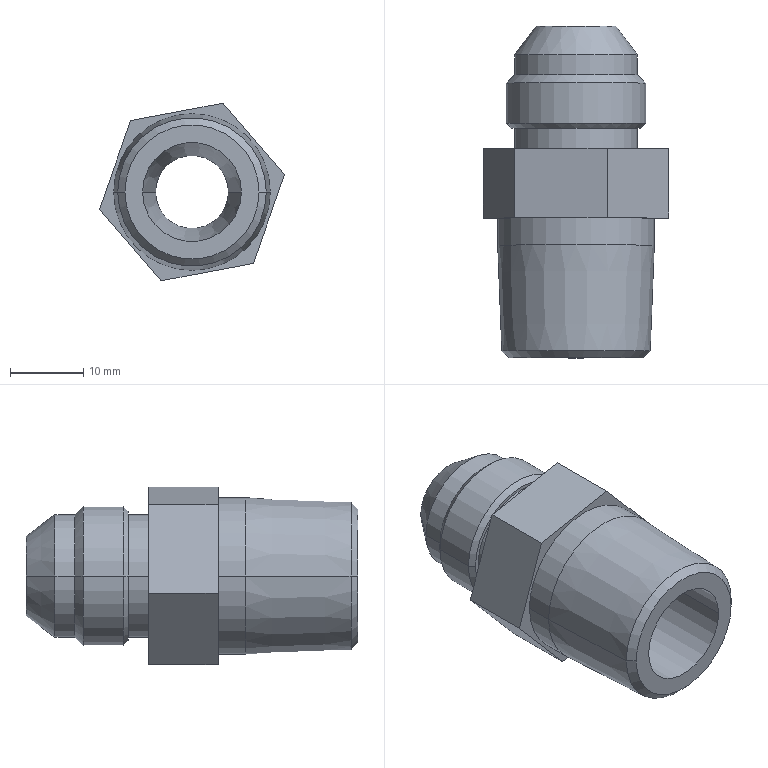Part | STEP file | 4-20.sldasm-Part-131 | 1 solid | 35 faces | box 25.216 x 45.212 x 24.222 mm | volume 9310 mm3 | cone 12 | cylinder 12 | plane 11 | commonest cylinder face diameters 9.931 x2 13.487 x2 16.662 x2 16.739 x2 19.009 x2 21.336 x2
STEP:
#1=CARTESIAN_POINT('',(133.988,509.63,44.));
#2=VERTEX_POINT('',#1);
#3=CARTESIAN_POINT('',(152.262,509.63,44.));
#4=VERTEX_POINT('',#3);
#5=CARTESIAN_POINT('',(143.125,509.63,44.));
#6=DIRECTION('',(0.,-1.,0.));
#7=DIRECTION('',(-1.,0.,0.));
#8=AXIS2_PLACEMENT_3D('',#5,#6,#7);
#9=CIRCLE('',#8,9.137);
#10=EDGE_CURVE('',#2,#4,#9,.T.);
#11=ORIENTED_EDGE('',*,*,#10,.F.);
#12=CARTESIAN_POINT('',(133.012,510.57,44.));
#13=VERTEX_POINT('',#12);
#14=CARTESIAN_POINT('',(133.988,509.63,44.));
#15=DIRECTION('',(-0.7206,0.6934,0.));
#16=VECTOR('',#15,1000.);
#17=LINE('',#14,#16);
#18=EDGE_CURVE('',#2,#13,#17,.T.);
#19=ORIENTED_EDGE('',*,*,#18,.T.);
#20=CARTESIAN_POINT('',(153.238,510.57,44.));
#21=VERTEX_POINT('',#20);
#22=CARTESIAN_POINT('',(143.125,510.57,44.));
#23=DIRECTION('',(0.,1.,0.));
#24=DIRECTION('',(-1.,0.,0.));
#25=AXIS2_PLACEMENT_3D('',#22,#23,#24);
#26=CIRCLE('',#25,10.113);
#27=EDGE_CURVE('',#21,#13,#26,.T.);
#28=ORIENTED_EDGE('',*,*,#27,.F.);
#29=CARTESIAN_POINT('',(152.262,509.63,44.));
#30=DIRECTION('',(0.7206,0.6934,0.));
#31=VECTOR('',#30,1000.);
#32=LINE('',#29,#31);
#33=EDGE_CURVE('',#4,#21,#32,.T.);
#34=ORIENTED_EDGE('',*,*,#33,.F.);
#35=EDGE_LOOP('',(#11,#19,#28,#34));
#36=FACE_OUTER_BOUND('',#35,.T.);
#37=CARTESIAN_POINT('',(143.125,509.63,44.));
#38=DIRECTION('',(0.,1.,0.));
#39=DIRECTION('',(1.,0.,0.));
#40=AXIS2_PLACEMENT_3D('',#37,#38,#39);
#41=CONICAL_SURFACE('',#40,9.137,0.8046);
#42=ADVANCED_FACE('',(#36),#41,.T.);
#43=CARTESIAN_POINT('',(134.756,548.213,44.));
#44=VERTEX_POINT('',#43);
#45=CARTESIAN_POINT('',(151.494,548.213,44.));
#46=VERTEX_POINT('',#45);
#47=CARTESIAN_POINT('',(143.125,548.213,44.));
#48=DIRECTION('',(0.,-1.,0.));
#49=DIRECTION('',(-1.,0.,0.));
#50=AXIS2_PLACEMENT_3D('',#47,#48,#49);
#51=CIRCLE('',#50,8.369);
#52=EDGE_CURVE('',#44,#46,#51,.T.);
#53=ORIENTED_EDGE('',*,*,#52,.T.);
#54=CARTESIAN_POINT('',(152.63,547.078,44.));
#55=VERTEX_POINT('',#54);
#56=CARTESIAN_POINT('',(152.63,547.078,44.));
#57=DIRECTION('',(0.7071,-0.7071,0.));
#58=VECTOR('',#57,1000.);
#59=LINE('',#56,#58);
#60=EDGE_CURVE('',#46,#55,#59,.T.);
#61=ORIENTED_EDGE('',*,*,#60,.T.);
#62=CARTESIAN_POINT('',(133.62,547.078,44.));
#63=VERTEX_POINT('',#62);
#64=CARTESIAN_POINT('',(143.125,547.078,44.));
#65=DIRECTION('',(0.,-1.,0.));
#66=DIRECTION('',(1.,0.,0.));
#67=AXIS2_PLACEMENT_3D('',#64,#65,#66);
#68=CIRCLE('',#67,9.505);
#69=EDGE_CURVE('',#63,#55,#68,.T.);
#70=ORIENTED_EDGE('',*,*,#69,.F.);
#71=CARTESIAN_POINT('',(133.62,547.078,44.));
#72=DIRECTION('',(-0.7071,-0.7071,0.));
#73=VECTOR('',#72,1000.);
#74=LINE('',#71,#73);
#75=EDGE_CURVE('',#44,#63,#74,.T.);
#76=ORIENTED_EDGE('',*,*,#75,.F.);
#77=EDGE_LOOP('',(#53,#61,#70,#76));
#78=FACE_OUTER_BOUND('',#77,.T.);
#79=CARTESIAN_POINT('',(143.125,547.078,44.));
#80=DIRECTION('',(0.,-1.,0.));
#81=DIRECTION('',(-1.,0.,0.));
#82=AXIS2_PLACEMENT_3D('',#79,#80,#81);
#83=CONICAL_SURFACE('',#82,9.505,0.7854);
#84=ADVANCED_FACE('',(#78),#83,.T.);
#85=CARTESIAN_POINT('',(134.298,540.923,44.));
#86=VERTEX_POINT('',#85);
#87=CARTESIAN_POINT('',(151.951,540.923,44.));
#88=VERTEX_POINT('',#87);
#89=CARTESIAN_POINT('',(143.125,540.923,44.));
#90=DIRECTION('',(0.,-1.,0.));
#91=DIRECTION('',(-1.,0.,0.));
#92=AXIS2_PLACEMENT_3D('',#89,#90,#91);
#93=CIRCLE('',#92,8.826);
#94=EDGE_CURVE('',#86,#88,#93,.T.);
#95=ORIENTED_EDGE('',*,*,#94,.F.);
#96=CARTESIAN_POINT('',(133.62,541.601,44.));
#97=VERTEX_POINT('',#96);
#98=CARTESIAN_POINT('',(134.298,540.923,44.));
#99=DIRECTION('',(-0.7071,0.7071,0.));
#100=VECTOR('',#99,1000.);
#101=LINE('',#98,#100);
#102=EDGE_CURVE('',#86,#97,#101,.T.);
#103=ORIENTED_EDGE('',*,*,#102,.T.);
#104=CARTESIAN_POINT('',(152.63,541.601,44.));
#105=VERTEX_POINT('',#104);
#106=CARTESIAN_POINT('',(143.125,541.601,44.));
#107=DIRECTION('',(0.,1.,0.));
#108=DIRECTION('',(-1.,0.,0.));
#109=AXIS2_PLACEMENT_3D('',#106,#107,#108);
#110=CIRCLE('',#109,9.505);
#111=EDGE_CURVE('',#105,#97,#110,.T.);
#112=ORIENTED_EDGE('',*,*,#111,.F.);
#113=CARTESIAN_POINT('',(151.951,540.923,44.));
#114=DIRECTION('',(0.7071,0.7071,0.));
#115=VECTOR('',#114,1000.);
#116=LINE('',#113,#115);
#117=EDGE_CURVE('',#88,#105,#116,.T.);
#118=ORIENTED_EDGE('',*,*,#117,.F.);
#119=EDGE_LOOP('',(#95,#103,#112,#118));
#120=FACE_OUTER_BOUND('',#119,.T.);
#121=CARTESIAN_POINT('',(143.125,540.923,44.));
#122=DIRECTION('',(0.,1.,0.));
#123=DIRECTION('',(1.,0.,0.));
#124=AXIS2_PLACEMENT_3D('',#121,#122,#123);
#125=CONICAL_SURFACE('',#124,8.826,0.7854);
#126=ADVANCED_FACE('',(#120),#125,.T.);
#127=ORIENTED_EDGE('',*,*,#27,.T.);
#128=CARTESIAN_POINT('',(132.457,525.,44.));
#129=VERTEX_POINT('',#128);
#130=CARTESIAN_POINT('',(133.048,509.63,44.));
#131=DIRECTION('',(-0.03843,0.9993,0.));
#132=VECTOR('',#131,1000.);
#133=LINE('',#130,#132);
#134=EDGE_CURVE('',#13,#129,#133,.T.);
#135=ORIENTED_EDGE('',*,*,#134,.T.);
#136=CARTESIAN_POINT('',(153.793,525.,44.));
#137=VERTEX_POINT('',#136);
#138=CARTESIAN_POINT('',(143.125,525.,44.));
#139=DIRECTION('',(0.,1.,0.));
#140=DIRECTION('',(-1.,0.,0.));
#141=AXIS2_PLACEMENT_3D('',#138,#139,#140);
#142=CIRCLE('',#141,10.668);
#143=EDGE_CURVE('',#137,#129,#142,.T.);
#144=ORIENTED_EDGE('',*,*,#143,.F.);
#145=CARTESIAN_POINT('',(153.202,509.63,44.));
#146=DIRECTION('',(0.03843,0.9993,0.));
#147=VECTOR('',#146,1000.);
#148=LINE('',#145,#147);
#149=EDGE_CURVE('',#21,#137,#148,.T.);
#150=ORIENTED_EDGE('',*,*,#149,.F.);
#151=EDGE_LOOP('',(#127,#135,#144,#150));
#152=FACE_OUTER_BOUND('',#151,.T.);
#153=CARTESIAN_POINT('',(143.125,509.63,44.));
#154=DIRECTION('',(0.,1.,0.));
#155=DIRECTION('',(1.,0.,0.));
#156=AXIS2_PLACEMENT_3D('',#153,#154,#155);
#157=CONICAL_SURFACE('',#156,10.077,0.03844);
#158=ADVANCED_FACE('',(#152),#157,.T.);
#159=CARTESIAN_POINT('',(134.794,540.923,44.));
#160=VERTEX_POINT('',#159);
#161=CARTESIAN_POINT('',(151.456,540.923,44.));
#162=VERTEX_POINT('',#161);
#163=CARTESIAN_POINT('',(143.125,540.923,44.));
#164=DIRECTION('',(0.,-1.,0.));
#165=DIRECTION('',(-1.,0.,0.));
#166=AXIS2_PLACEMENT_3D('',#163,#164,#165);
#167=CIRCLE('',#166,8.331);
#168=EDGE_CURVE('',#160,#162,#167,.T.);
#169=ORIENTED_EDGE('',*,*,#168,.T.);
#170=CARTESIAN_POINT('',(151.456,538.155,44.));
#171=VERTEX_POINT('',#170);
#172=CARTESIAN_POINT('',(151.456,420.38,44.));
#173=DIRECTION('',(0.,-1.,0.));
#174=VECTOR('',#173,1000.);
#175=LINE('',#172,#174);
#176=EDGE_CURVE('',#162,#171,#175,.T.);
#177=ORIENTED_EDGE('',*,*,#176,.T.);
#178=CARTESIAN_POINT('',(134.794,538.155,44.));
#179=VERTEX_POINT('',#178);
#180=CARTESIAN_POINT('',(143.125,538.155,44.));
#181=DIRECTION('',(0.,-1.,0.));
#182=DIRECTION('',(-1.,0.,0.));
#183=AXIS2_PLACEMENT_3D('',#180,#181,#182);
#184=CIRCLE('',#183,8.331);
#185=EDGE_CURVE('',#179,#171,#184,.T.);
#186=ORIENTED_EDGE('',*,*,#185,.F.);
#187=CARTESIAN_POINT('',(134.794,420.38,44.));
#188=DIRECTION('',(0.,-1.,0.));
#189=VECTOR('',#188,1000.);
#190=LINE('',#187,#189);
#191=EDGE_CURVE('',#160,#179,#190,.T.);
#192=ORIENTED_EDGE('',*,*,#191,.F.);
#193=EDGE_LOOP('',(#169,#177,#186,#192));
#194=FACE_OUTER_BOUND('',#193,.T.);
#195=CARTESIAN_POINT('',(143.125,420.38,44.));
#196=DIRECTION('',(0.,-1.,0.));
#197=DIRECTION('',(-1.,0.,0.));
#198=AXIS2_PLACEMENT_3D('',#195,#196,#197);
#199=CYLINDRICAL_SURFACE('',#198,8.331);
#200=ADVANCED_FACE('',(#194),#199,.T.);
#201=CARTESIAN_POINT('',(132.457,528.68,44.));
#202=VERTEX_POINT('',#201);
#203=CARTESIAN_POINT('',(153.793,528.68,44.));
#204=VERTEX_POINT('',#203);
#205=CARTESIAN_POINT('',(143.125,528.68,44.));
#206=DIRECTION('',(0.,-1.,0.));
#207=DIRECTION('',(-1.,0.,0.));
#208=AXIS2_PLACEMENT_3D('',#205,#206,#207);
#209=CIRCLE('',#208,10.668);
#210=EDGE_CURVE('',#202,#204,#209,.T.);
#211=ORIENTED_EDGE('',*,*,#210,.T.);
#212=CARTESIAN_POINT('',(153.793,420.38,44.));
#213=DIRECTION('',(0.,-1.,0.));
#214=VECTOR('',#213,1000.);
#215=LINE('',#212,#214);
#216=EDGE_CURVE('',#204,#137,#215,.T.);
#217=ORIENTED_EDGE('',*,*,#216,.T.);
#218=ORIENTED_EDGE('',*,*,#143,.T.);
#219=CARTESIAN_POINT('',(132.457,420.38,44.));
#220=DIRECTION('',(0.,-1.,0.));
#221=VECTOR('',#220,1000.);
#222=LINE('',#219,#221);
#223=EDGE_CURVE('',#202,#129,#222,.T.);
#224=ORIENTED_EDGE('',*,*,#223,.F.);
#225=EDGE_LOOP('',(#211,#217,#218,#224));
#226=FACE_OUTER_BOUND('',#225,.T.);
#227=CARTESIAN_POINT('',(143.125,420.38,44.));
#228=DIRECTION('',(0.,-1.,0.));
#229=DIRECTION('',(-1.,0.,0.));
#230=AXIS2_PLACEMENT_3D('',#227,#228,#229);
#231=CYLINDRICAL_SURFACE('',#230,10.668);
#232=ADVANCED_FACE('',(#226),#231,.T.);
#233=CARTESIAN_POINT('',(149.869,528.68,44.));
#234=VERTEX_POINT('',#233);
#235=CARTESIAN_POINT('',(136.381,528.68,44.));
#236=VERTEX_POINT('',#235);
#237=CARTESIAN_POINT('',(143.125,528.68,44.));
#238=DIRECTION('',(0.,-1.,0.));
#239=DIRECTION('',(-1.,0.,0.));
#240=AXIS2_PLACEMENT_3D('',#237,#238,#239);
#241=CIRCLE('',#240,6.744);
#242=EDGE_CURVE('',#234,#236,#241,.T.);
#243=ORIENTED_EDGE('',*,*,#242,.F.);
#244=CARTESIAN_POINT('',(149.869,509.63,44.));
#245=VERTEX_POINT('',#244);
#246=CARTESIAN_POINT('',(149.869,420.38,44.));
#247=DIRECTION('',(0.,-1.,0.));
#248=VECTOR('',#247,1000.);
#249=LINE('',#246,#248);
#250=EDGE_CURVE('',#234,#245,#249,.T.);
#251=ORIENTED_EDGE('',*,*,#250,.T.);
#252=CARTESIAN_POINT('',(136.381,509.63,44.));
#253=VERTEX_POINT('',#252);
#254=CARTESIAN_POINT('',(143.125,509.63,44.));
#255=DIRECTION('',(0.,-1.,0.));
#256=DIRECTION('',(-1.,0.,0.));
#257=AXIS2_PLACEMENT_3D('',#254,#255,#256);
#258=CIRCLE('',#257,6.744);
#259=EDGE_CURVE('',#245,#253,#258,.T.);
#260=ORIENTED_EDGE('',*,*,#259,.T.);
#261=CARTESIAN_POINT('',(136.381,420.38,44.));
#262=DIRECTION('',(0.,-1.,0.));
#263=VECTOR('',#262,1000.);
#264=LINE('',#261,#263);
#265=EDGE_CURVE('',#236,#253,#264,.T.);
#266=ORIENTED_EDGE('',*,*,#265,.F.);
#267=EDGE_LOOP('',(#243,#251,#260,#266));
#268=FACE_OUTER_BOUND('',#267,.T.);
#269=CARTESIAN_POINT('',(143.125,420.38,44.));
#270=DIRECTION('',(0.,-1.,0.));
#271=DIRECTION('',(-1.,0.,0.));
#272=AXIS2_PLACEMENT_3D('',#269,#270,#271);
#273=CYLINDRICAL_SURFACE('',#272,6.744);
#274=ADVANCED_FACE('',(#268),#273,.F.);
#275=CARTESIAN_POINT('',(148.091,538.155,44.));
#276=VERTEX_POINT('',#275);
#277=CARTESIAN_POINT('',(138.159,538.155,44.));
#278=VERTEX_POINT('',#277);
#279=CARTESIAN_POINT('',(143.125,538.155,44.));
#280=DIRECTION('',(0.,-1.,0.));
#281=DIRECTION('',(-1.,0.,0.));
#282=AXIS2_PLACEMENT_3D('',#279,#280,#281);
#283=CIRCLE('',#282,4.966);
#284=EDGE_CURVE('',#276,#278,#283,.T.);
#285=ORIENTED_EDGE('',*,*,#284,.F.);
#286=CARTESIAN_POINT('',(148.091,538.155,44.));
#287=DIRECTION('',(0.1844,-0.9828,0.));
#288=VECTOR('',#287,1000.);
#289=LINE('',#286,#288);
#290=EDGE_CURVE('',#276,#234,#289,.T.);
#291=ORIENTED_EDGE('',*,*,#290,.T.);
#292=ORIENTED_EDGE('',*,*,#242,.T.);
#293=CARTESIAN_POINT('',(138.159,538.155,44.));
#294=DIRECTION('',(-0.1844,-0.9828,0.));
#295=VECTOR('',#294,1000.);
#296=LINE('',#293,#295);
#297=EDGE_CURVE('',#278,#236,#296,.T.);
#298=ORIENTED_EDGE('',*,*,#297,.F.);
#299=EDGE_LOOP('',(#285,#291,#292,#298));
#300=FACE_OUTER_BOUND('',#299,.T.);
#301=CARTESIAN_POINT('',(143.125,538.155,44.));
#302=DIRECTION('',(0.,-1.,0.));
#303=DIRECTION('',(-1.,0.,0.));
#304=AXIS2_PLACEMENT_3D('',#301,#302,#303);
#305=CONICAL_SURFACE('',#304,4.966,0.1855);
#306=ADVANCED_FACE('',(#300),#305,.F.);
#307=CARTESIAN_POINT('',(148.091,554.842,44.));
#308=VERTEX_POINT('',#307);
#309=CARTESIAN_POINT('',(138.159,554.842,44.));
#310=VERTEX_POINT('',#309);
#311=CARTESIAN_POINT('',(143.125,554.842,44.));
#312=DIRECTION('',(0.,-1.,0.));
#313=DIRECTION('',(-1.,0.,0.));
#314=AXIS2_PLACEMENT_3D('',#311,#312,#313);
#315=CIRCLE('',#314,4.966);
#316=EDGE_CURVE('',#308,#310,#315,.T.);
#317=ORIENTED_EDGE('',*,*,#316,.F.);
#318=CARTESIAN_POINT('',(148.091,420.38,44.));
#319=DIRECTION('',(0.,-1.,0.));
#320=VECTOR('',#319,1000.);
#321=LINE('',#318,#320);
#322=EDGE_CURVE('',#308,#276,#321,.T.);
#323=ORIENTED_EDGE('',*,*,#322,.T.);
#324=ORIENTED_EDGE('',*,*,#284,.T.);
#325=CARTESIAN_POINT('',(138.159,420.38,44.));
#326=DIRECTION('',(0.,-1.,0.));
#327=VECTOR('',#326,1000.);
#328=LINE('',#325,#327);
#329=EDGE_CURVE('',#310,#278,#328,.T.);
#330=ORIENTED_EDGE('',*,*,#329,.F.);
#331=EDGE_LOOP('',(#317,#323,#324,#330));
#332=FACE_OUTER_BOUND('',#331,.T.);
#333=CARTESIAN_POINT('',(143.125,420.38,44.));
#334=DIRECTION('',(0.,-1.,0.));
#335=DIRECTION('',(-1.,0.,0.));
#336=AXIS2_PLACEMENT_3D('',#333,#334,#335);
#337=CYLINDRICAL_SURFACE('',#336,4.966);
#338=ADVANCED_FACE('',(#332),#337,.F.);
#339=CARTESIAN_POINT('',(137.677,554.842,44.));
#340=VERTEX_POINT('',#339);
#341=CARTESIAN_POINT('',(148.573,554.842,44.));
#342=VERTEX_POINT('',#341);
#343=CARTESIAN_POINT('',(143.125,554.842,44.));
#344=DIRECTION('',(0.,-1.,0.));
#345=DIRECTION('',(-1.,0.,0.));
#346=AXIS2_PLACEMENT_3D('',#343,#344,#345);
#347=CIRCLE('',#346,5.448);
#348=EDGE_CURVE('',#340,#342,#347,.T.);
#349=ORIENTED_EDGE('',*,*,#348,.T.);
#350=CARTESIAN_POINT('',(151.494,550.916,44.));
#351=VERTEX_POINT('',#350);
#352=CARTESIAN_POINT('',(151.494,550.916,44.));
#353=DIRECTION('',(0.5968,-0.8024,0.));
#354=VECTOR('',#353,1000.);
#355=LINE('',#352,#354);
#356=EDGE_CURVE('',#342,#351,#355,.T.);
#357=ORIENTED_EDGE('',*,*,#356,.T.);
#358=CARTESIAN_POINT('',(134.756,550.916,44.));
#359=VERTEX_POINT('',#358);
#360=CARTESIAN_POINT('',(143.125,550.916,44.));
#361=DIRECTION('',(0.,-1.,0.));
#362=DIRECTION('',(-1.,0.,0.));
#363=AXIS2_PLACEMENT_3D('',#360,#361,#362);
#364=CIRCLE('',#363,8.369);
#365=EDGE_CURVE('',#359,#351,#364,.T.);
#366=ORIENTED_EDGE('',*,*,#365,.F.);
#367=CARTESIAN_POINT('',(134.756,550.916,44.));
#368=DIRECTION('',(-0.5968,-0.8024,0.));
#369=VECTOR('',#368,1000.);
#370=LINE('',#367,#369);
#371=EDGE_CURVE('',#340,#359,#370,.T.);
#372=ORIENTED_EDGE('',*,*,#371,.F.);
#373=EDGE_LOOP('',(#349,#357,#366,#372));
#374=FACE_OUTER_BOUND('',#373,.T.);
#375=CARTESIAN_POINT('',(143.125,550.916,44.));
#376=DIRECTION('',(0.,-1.,0.));
#377=DIRECTION('',(-1.,0.,0.));
#378=AXIS2_PLACEMENT_3D('',#375,#376,#377);
#379=CONICAL_SURFACE('',#378,8.369,0.6396);
#380=ADVANCED_FACE('',(#374),#379,.T.);
#381=ORIENTED_EDGE('',*,*,#365,.T.);
#382=CARTESIAN_POINT('',(151.494,420.38,44.));
#383=DIRECTION('',(0.,-1.,0.));
#384=VECTOR('',#383,1000.);
#385=LINE('',#382,#384);
#386=EDGE_CURVE('',#351,#46,#385,.T.);
#387=ORIENTED_EDGE('',*,*,#386,.T.);
#388=ORIENTED_EDGE('',*,*,#52,.F.);
#389=CARTESIAN_POINT('',(134.756,420.38,44.));
#390=DIRECTION('',(0.,-1.,0.));
#391=VECTOR('',#390,1000.);
#392=LINE('',#389,#391);
#393=EDGE_CURVE('',#359,#44,#392,.T.);
#394=ORIENTED_EDGE('',*,*,#393,.F.);
#395=EDGE_LOOP('',(#381,#387,#388,#394));
#396=FACE_OUTER_BOUND('',#395,.T.);
#397=CARTESIAN_POINT('',(143.125,420.38,44.));
#398=DIRECTION('',(0.,-1.,0.));
#399=DIRECTION('',(-1.,0.,0.));
#400=AXIS2_PLACEMENT_3D('',#397,#398,#399);
#401=CYLINDRICAL_SURFACE('',#400,8.369);
#402=ADVANCED_FACE('',(#396),#401,.T.);
#403=ORIENTED_EDGE('',*,*,#69,.T.);
#404=CARTESIAN_POINT('',(152.63,420.38,44.));
#405=DIRECTION('',(0.,-1.,0.));
#406=VECTOR('',#405,1000.);
#407=LINE('',#404,#406);
#408=EDGE_CURVE('',#55,#105,#407,.T.);
#409=ORIENTED_EDGE('',*,*,#408,.T.);
#410=ORIENTED_EDGE('',*,*,#111,.T.);
#411=CARTESIAN_POINT('',(133.62,420.38,44.));
#412=DIRECTION('',(0.,-1.,0.));
#413=VECTOR('',#412,1000.);
#414=LINE('',#411,#413);
#415=EDGE_CURVE('',#63,#97,#414,.T.);
#416=ORIENTED_EDGE('',*,*,#415,.F.);
#417=EDGE_LOOP('',(#403,#409,#410,#416));
#418=FACE_OUTER_BOUND('',#417,.T.);
#419=CARTESIAN_POINT('',(143.125,420.38,44.));
#420=DIRECTION('',(0.,-1.,0.));
#421=DIRECTION('',(-1.,0.,0.));
#422=AXIS2_PLACEMENT_3D('',#419,#420,#421);
#423=CYLINDRICAL_SURFACE('',#422,9.505);
#424=ADVANCED_FACE('',(#418),#423,.T.);
#425=ORIENTED_EDGE('',*,*,#210,.F.);
#426=CARTESIAN_POINT('',(143.125,528.68,44.));
#427=DIRECTION('',(0.,-1.,0.));
#428=DIRECTION('',(-1.,0.,0.));
#429=AXIS2_PLACEMENT_3D('',#426,#427,#428);
#430=CIRCLE('',#429,10.668);
#431=EDGE_CURVE('',#204,#202,#430,.T.);
#432=ORIENTED_EDGE('',*,*,#431,.F.);
#433=EDGE_LOOP('',(#425,#432));
#434=FACE_BOUND('',#433,.T.);
#435=CARTESIAN_POINT('',(147.365,528.68,56.111));
#436=VERTEX_POINT('',#435);
#437=CARTESIAN_POINT('',(134.756,528.68,53.727));
#438=VERTEX_POINT('',#437);
#439=CARTESIAN_POINT('',(139.113,528.68,54.551));
#440=DIRECTION('',(-0.9826,0.,-0.1858));
#441=VECTOR('',#440,1000.);
#442=LINE('',#439,#441);
#443=EDGE_CURVE('',#436,#438,#442,.T.);
#444=ORIENTED_EDGE('',*,*,#443,.T.);
#445=CARTESIAN_POINT('',(130.517,528.68,41.616));
#446=VERTEX_POINT('',#445);
#447=CARTESIAN_POINT('',(129.31,528.68,38.168));
#448=DIRECTION('',(-0.3304,0.,-0.9438));
#449=VECTOR('',#448,1000.);
#450=LINE('',#447,#449);
#451=EDGE_CURVE('',#438,#446,#450,.T.);
#452=ORIENTED_EDGE('',*,*,#451,.T.);
#453=CARTESIAN_POINT('',(138.885,528.68,31.889));
#454=VERTEX_POINT('',#453);
#455=CARTESIAN_POINT('',(139.975,528.68,30.622));
#456=DIRECTION('',(0.6522,0.,-0.7581));
#457=VECTOR('',#456,1000.);
#458=LINE('',#455,#457);
#459=EDGE_CURVE('',#446,#454,#458,.T.);
#460=ORIENTED_EDGE('',*,*,#459,.T.);
#461=CARTESIAN_POINT('',(151.494,528.68,34.273));
#462=VERTEX_POINT('',#461);
#463=CARTESIAN_POINT('',(143.242,528.68,32.713));
#464=DIRECTION('',(0.9826,0.,0.1858));
#465=VECTOR('',#464,1000.);
#466=LINE('',#463,#465);
#467=EDGE_CURVE('',#454,#462,#466,.T.);
#468=ORIENTED_EDGE('',*,*,#467,.T.);
#469=CARTESIAN_POINT('',(155.733,528.68,46.384));
#470=VERTEX_POINT('',#469);
#471=CARTESIAN_POINT('',(150.287,528.68,30.825));
#472=DIRECTION('',(0.3304,0.,0.9438));
#473=VECTOR('',#472,1000.);
#474=LINE('',#471,#473);
#475=EDGE_CURVE('',#462,#470,#474,.T.);
#476=ORIENTED_EDGE('',*,*,#475,.T.);
#477=CARTESIAN_POINT('',(156.823,528.68,45.117));
#478=DIRECTION('',(-0.6522,0.,0.7581));
#479=VECTOR('',#478,1000.);
#480=LINE('',#477,#479);
#481=EDGE_CURVE('',#470,#436,#480,.T.);
#482=ORIENTED_EDGE('',*,*,#481,.T.);
#483=EDGE_LOOP('',(#444,#452,#460,#468,#476,#482));
#484=FACE_OUTER_BOUND('',#483,.T.);
#485=CARTESIAN_POINT('',(143.125,528.68,33.332));
#486=DIRECTION('',(0.,-1.,0.));
#487=DIRECTION('',(-1.,0.,0.));
#488=AXIS2_PLACEMENT_3D('',#485,#486,#487);
#489=PLANE('',#488);
#490=ADVANCED_FACE('',(#434,#484),#489,.T.);
#491=ORIENTED_EDGE('',*,*,#185,.T.);
#492=CARTESIAN_POINT('',(143.125,538.155,44.));
#493=DIRECTION('',(0.,-1.,0.));
#494=DIRECTION('',(-1.,0.,0.));
#495=AXIS2_PLACEMENT_3D('',#492,#493,#494);
#496=CIRCLE('',#495,8.331);
#497=EDGE_CURVE('',#171,#179,#496,.T.);
#498=ORIENTED_EDGE('',*,*,#497,.T.);
#499=EDGE_LOOP('',(#491,#498));
#500=FACE_BOUND('',#499,.T.);
#501=CARTESIAN_POINT('',(130.517,538.155,41.616));
#502=VERTEX_POINT('',#501);
#503=CARTESIAN_POINT('',(138.885,538.155,31.889));
#504=VERTEX_POINT('',#503);
#505=CARTESIAN_POINT('',(130.517,538.155,41.616));
#506=DIRECTION('',(0.6522,0.,-0.7581));
#507=VECTOR('',#506,1000.);
#508=LINE('',#505,#507);
#509=EDGE_CURVE('',#502,#504,#508,.T.);
#510=ORIENTED_EDGE('',*,*,#509,.F.);
#511=CARTESIAN_POINT('',(134.756,538.155,53.727));
#512=VERTEX_POINT('',#511);
#513=CARTESIAN_POINT('',(134.756,538.155,53.727));
#514=DIRECTION('',(-0.3304,0.,-0.9438));
#515=VECTOR('',#514,1000.);
#516=LINE('',#513,#515);
#517=EDGE_CURVE('',#512,#502,#516,.T.);
#518=ORIENTED_EDGE('',*,*,#517,.F.);
#519=CARTESIAN_POINT('',(147.365,538.155,56.111));
#520=VERTEX_POINT('',#519);
#521=CARTESIAN_POINT('',(147.365,538.155,56.111));
#522=DIRECTION('',(-0.9826,0.,-0.1858));
#523=VECTOR('',#522,1000.);
#524=LINE('',#521,#523);
#525=EDGE_CURVE('',#520,#512,#524,.T.);
#526=ORIENTED_EDGE('',*,*,#525,.F.);
#527=CARTESIAN_POINT('',(155.733,538.155,46.384));
#528=VERTEX_POINT('',#527);
#529=CARTESIAN_POINT('',(155.733,538.155,46.384));
#530=DIRECTION('',(-0.6522,0.,0.7581));
#531=VECTOR('',#530,1000.);
#532=LINE('',#529,#531);
#533=EDGE_CURVE('',#528,#520,#532,.T.);
#534=ORIENTED_EDGE('',*,*,#533,.F.);
#535=CARTESIAN_POINT('',(151.494,538.155,34.273));
#536=VERTEX_POINT('',#535);
#537=CARTESIAN_POINT('',(151.494,538.155,34.273));
#538=DIRECTION('',(0.3304,0.,0.9438));
#539=VECTOR('',#538,1000.);
#540=LINE('',#537,#539);
#541=EDGE_CURVE('',#536,#528,#540,.T.);
#542=ORIENTED_EDGE('',*,*,#541,.F.);
#543=CARTESIAN_POINT('',(138.885,538.155,31.889));
#544=DIRECTION('',(0.9826,0.,0.1858));
#545=VECTOR('',#544,1000.);
#546=LINE('',#543,#545);
#547=EDGE_CURVE('',#504,#536,#546,.T.);
#548=ORIENTED_EDGE('',*,*,#547,.F.);
#549=EDGE_LOOP('',(#510,#518,#526,#534,#542,#548));
#550=FACE_OUTER_BOUND('',#549,.T.);
#551=CARTESIAN_POINT('',(143.125,538.155,31.168));
#552=DIRECTION('',(0.,1.,0.));
#553=DIRECTION('',(1.,0.,0.));
#554=AXIS2_PLACEMENT_3D('',#551,#552,#553);
#555=PLANE('',#554);
#556=ADVANCED_FACE('',(#500,#550),#555,.T.);
#557=CARTESIAN_POINT('',(143.125,540.923,44.));
#558=DIRECTION('',(0.,-1.,0.));
#559=DIRECTION('',(-1.,0.,0.));
#560=AXIS2_PLACEMENT_3D('',#557,#558,#559);
#561=CIRCLE('',#560,8.826);
#562=EDGE_CURVE('',#88,#86,#561,.T.);
#563=ORIENTED_EDGE('',*,*,#562,.T.);
#564=ORIENTED_EDGE('',*,*,#94,.T.);
#565=EDGE_LOOP('',(#563,#564));
#566=FACE_OUTER_BOUND('',#565,.T.);
#567=ORIENTED_EDGE('',*,*,#168,.F.);
#568=CARTESIAN_POINT('',(143.125,540.923,44.));
#569=DIRECTION('',(0.,-1.,0.));
#570=DIRECTION('',(-1.,0.,0.));
#571=AXIS2_PLACEMENT_3D('',#568,#569,#570);
#572=CIRCLE('',#571,8.331);
#573=EDGE_CURVE('',#162,#160,#572,.T.);
#574=ORIENTED_EDGE('',*,*,#573,.F.);
#575=EDGE_LOOP('',(#567,#574));
#576=FACE_BOUND('',#575,.T.);
#577=CARTESIAN_POINT('',(143.125,540.923,35.669));
#578=DIRECTION('',(0.,-1.,0.));
#579=DIRECTION('',(-1.,0.,0.));
#580=AXIS2_PLACEMENT_3D('',#577,#578,#579);
#581=PLANE('',#580);
#582=ADVANCED_FACE('',(#566,#576),#581,.T.);
#583=ORIENTED_EDGE('',*,*,#408,.F.);
#584=CARTESIAN_POINT('',(143.125,547.078,44.));
#585=DIRECTION('',(0.,-1.,0.));
#586=DIRECTION('',(1.,0.,0.));
#587=AXIS2_PLACEMENT_3D('',#584,#585,#586);
#588=CIRCLE('',#587,9.505);
#589=EDGE_CURVE('',#55,#63,#588,.T.);
#590=ORIENTED_EDGE('',*,*,#589,.T.);
#591=ORIENTED_EDGE('',*,*,#415,.T.);
#592=CARTESIAN_POINT('',(143.125,541.601,44.));
#593=DIRECTION('',(0.,1.,0.));
#594=DIRECTION('',(-1.,0.,0.));
#595=AXIS2_PLACEMENT_3D('',#592,#593,#594);
#596=CIRCLE('',#595,9.505);
#597=EDGE_CURVE('',#97,#105,#596,.T.);
#598=ORIENTED_EDGE('',*,*,#597,.T.);
#599=EDGE_LOOP('',(#583,#590,#591,#598));
#600=FACE_OUTER_BOUND('',#599,.T.);
#601=CARTESIAN_POINT('',(143.125,420.38,44.));
#602=DIRECTION('',(0.,-1.,0.));
#603=DIRECTION('',(-1.,0.,0.));
#604=AXIS2_PLACEMENT_3D('',#601,#602,#603);
#605=CYLINDRICAL_SURFACE('',#604,9.505);
#606=ADVANCED_FACE('',(#600),#605,.T.);
#607=ORIENTED_EDGE('',*,*,#386,.F.);
#608=CARTESIAN_POINT('',(143.125,550.916,44.));
#609=DIRECTION('',(0.,-1.,0.));
#610=DIRECTION('',(-1.,0.,0.));
#611=AXIS2_PLACEMENT_3D('',#608,#609,#610);
#612=CIRCLE('',#611,8.369);
#613=EDGE_CURVE('',#351,#359,#612,.T.);
#614=ORIENTED_EDGE('',*,*,#613,.T.);
#615=ORIENTED_EDGE('',*,*,#393,.T.);
#616=CARTESIAN_POINT('',(143.125,548.213,44.));
#617=DIRECTION('',(0.,-1.,0.));
#618=DIRECTION('',(-1.,0.,0.));
#619=AXIS2_PLACEMENT_3D('',#616,#617,#618);
#620=CIRCLE('',#619,8.369);
#621=EDGE_CURVE('',#46,#44,#620,.T.);
#622=ORIENTED_EDGE('',*,*,#621,.F.);
#623=EDGE_LOOP('',(#607,#614,#615,#622));
#624=FACE_OUTER_BOUND('',#623,.T.);
#625=CARTESIAN_POINT('',(143.125,420.38,44.));
#626=DIRECTION('',(0.,-1.,0.));
#627=DIRECTION('',(-1.,0.,0.));
#628=AXIS2_PLACEMENT_3D('',#625,#626,#627);
#629=CYLINDRICAL_SURFACE('',#628,8.369);
#630=ADVANCED_FACE('',(#624),#629,.T.);
#631=ORIENTED_EDGE('',*,*,#356,.F.);
#632=CARTESIAN_POINT('',(143.125,554.842,44.));
#633=DIRECTION('',(0.,-1.,0.));
#634=DIRECTION('',(-1.,0.,0.));
#635=AXIS2_PLACEMENT_3D('',#632,#633,#634);
#636=CIRCLE('',#635,5.448);
#637=EDGE_CURVE('',#342,#340,#636,.T.);
#638=ORIENTED_EDGE('',*,*,#637,.T.);
#639=ORIENTED_EDGE('',*,*,#371,.T.);
#640=ORIENTED_EDGE('',*,*,#613,.F.);
#641=EDGE_LOOP('',(#631,#638,#639,#640));
#642=FACE_OUTER_BOUND('',#641,.T.);
#643=CARTESIAN_POINT('',(143.125,550.916,44.));
#644=DIRECTION('',(0.,-1.,0.));
#645=DIRECTION('',(-1.,0.,0.));
#646=AXIS2_PLACEMENT_3D('',#643,#644,#645);
#647=CONICAL_SURFACE('',#646,8.369,0.6396);
#648=ADVANCED_FACE('',(#642),#647,.T.);
#649=CARTESIAN_POINT('',(143.125,554.842,44.));
#650=DIRECTION('',(0.,-1.,0.));
#651=DIRECTION('',(-1.,0.,0.));
#652=AXIS2_PLACEMENT_3D('',#649,#650,#651);
#653=CIRCLE('',#652,4.966);
#654=EDGE_CURVE('',#310,#308,#653,.T.);
#655=ORIENTED_EDGE('',*,*,#654,.T.);
#656=ORIENTED_EDGE('',*,*,#316,.T.);
#657=EDGE_LOOP('',(#655,#656));
#658=FACE_BOUND('',#657,.T.);
#659=ORIENTED_EDGE('',*,*,#348,.F.);
#660=ORIENTED_EDGE('',*,*,#637,.F.);
#661=EDGE_LOOP('',(#659,#660));
#662=FACE_OUTER_BOUND('',#661,.T.);
#663=CARTESIAN_POINT('',(143.125,554.842,38.552));
#664=DIRECTION('',(0.,1.,0.));
#665=DIRECTION('',(1.,0.,0.));
#666=AXIS2_PLACEMENT_3D('',#663,#664,#665);
#667=PLANE('',#666);
#668=ADVANCED_FACE('',(#658,#662),#667,.T.);
#669=ORIENTED_EDGE('',*,*,#322,.F.);
#670=ORIENTED_EDGE('',*,*,#654,.F.);
#671=ORIENTED_EDGE('',*,*,#329,.T.);
#672=CARTESIAN_POINT('',(143.125,538.155,44.));
#673=DIRECTION('',(0.,-1.,0.));
#674=DIRECTION('',(-1.,0.,0.));
#675=AXIS2_PLACEMENT_3D('',#672,#673,#674);
#676=CIRCLE('',#675,4.966);
#677=EDGE_CURVE('',#278,#276,#676,.T.);
#678=ORIENTED_EDGE('',*,*,#677,.T.);
#679=EDGE_LOOP('',(#669,#670,#671,#678));
#680=FACE_OUTER_BOUND('',#679,.T.);
#681=CARTESIAN_POINT('',(143.125,420.38,44.));
#682=DIRECTION('',(0.,-1.,0.));
#683=DIRECTION('',(-1.,0.,0.));
#684=AXIS2_PLACEMENT_3D('',#681,#682,#683);
#685=CYLINDRICAL_SURFACE('',#684,4.966);
#686=ADVANCED_FACE('',(#680),#685,.F.);
#687=ORIENTED_EDGE('',*,*,#290,.F.);
#688=ORIENTED_EDGE('',*,*,#677,.F.);
#689=ORIENTED_EDGE('',*,*,#297,.T.);
#690=CARTESIAN_POINT('',(143.125,528.68,44.));
#691=DIRECTION('',(0.,-1.,0.));
#692=DIRECTION('',(-1.,0.,0.));
#693=AXIS2_PLACEMENT_3D('',#690,#691,#692);
#694=CIRCLE('',#693,6.744);
#695=EDGE_CURVE('',#236,#234,#694,.T.);
#696=ORIENTED_EDGE('',*,*,#695,.T.);
#697=EDGE_LOOP('',(#687,#688,#689,#696));
#698=FACE_OUTER_BOUND('',#697,.T.);
#699=CARTESIAN_POINT('',(143.125,538.155,44.));
#700=DIRECTION('',(0.,-1.,0.));
#701=DIRECTION('',(-1.,0.,0.));
#702=AXIS2_PLACEMENT_3D('',#699,#700,#701);
#703=CONICAL_SURFACE('',#702,4.966,0.1855);
#704=ADVANCED_FACE('',(#698),#703,.F.);
#705=ORIENTED_EDGE('',*,*,#250,.F.);
#706=ORIENTED_EDGE('',*,*,#695,.F.);
#707=ORIENTED_EDGE('',*,*,#265,.T.);
#708=CARTESIAN_POINT('',(143.125,509.63,44.));
#709=DIRECTION('',(0.,-1.,0.));
#710=DIRECTION('',(-1.,0.,0.));
#711=AXIS2_PLACEMENT_3D('',#708,#709,#710);
#712=CIRCLE('',#711,6.744);
#713=EDGE_CURVE('',#253,#245,#712,.T.);
#714=ORIENTED_EDGE('',*,*,#713,.T.);
#715=EDGE_LOOP('',(#705,#706,#707,#714));
#716=FACE_OUTER_BOUND('',#715,.T.);
#717=CARTESIAN_POINT('',(143.125,420.38,44.));
#718=DIRECTION('',(0.,-1.,0.));
#719=DIRECTION('',(-1.,0.,0.));
#720=AXIS2_PLACEMENT_3D('',#717,#718,#719);
#721=CYLINDRICAL_SURFACE('',#720,6.744);
#722=ADVANCED_FACE('',(#716),#721,.F.);
#723=CARTESIAN_POINT('',(143.125,509.63,44.));
#724=DIRECTION('',(0.,-1.,0.));
#725=DIRECTION('',(-1.,0.,0.));
#726=AXIS2_PLACEMENT_3D('',#723,#724,#725);
#727=CIRCLE('',#726,9.137);
#728=EDGE_CURVE('',#4,#2,#727,.T.);
#729=ORIENTED_EDGE('',*,*,#728,.T.);
#730=ORIENTED_EDGE('',*,*,#10,.T.);
#731=EDGE_LOOP('',(#729,#730));
#732=FACE_OUTER_BOUND('',#731,.T.);
#733=ORIENTED_EDGE('',*,*,#713,.F.);
#734=ORIENTED_EDGE('',*,*,#259,.F.);
#735=EDGE_LOOP('',(#733,#734));
#736=FACE_BOUND('',#735,.T.);
#737=CARTESIAN_POINT('',(143.125,509.63,37.256));
#738=DIRECTION('',(0.,-1.,0.));
#739=DIRECTION('',(-1.,0.,0.));
#740=AXIS2_PLACEMENT_3D('',#737,#738,#739);
#741=PLANE('',#740);
#742=ADVANCED_FACE('',(#732,#736),#741,.T.);
#743=ORIENTED_EDGE('',*,*,#216,.F.);
#744=ORIENTED_EDGE('',*,*,#431,.T.);
#745=ORIENTED_EDGE('',*,*,#223,.T.);
#746=CARTESIAN_POINT('',(143.125,525.,44.));
#747=DIRECTION('',(0.,1.,0.));
#748=DIRECTION('',(-1.,0.,0.));
#749=AXIS2_PLACEMENT_3D('',#746,#747,#748);
#750=CIRCLE('',#749,10.668);
#751=EDGE_CURVE('',#129,#137,#750,.T.);
#752=ORIENTED_EDGE('',*,*,#751,.T.);
#753=EDGE_LOOP('',(#743,#744,#745,#752));
#754=FACE_OUTER_BOUND('',#753,.T.);
#755=CARTESIAN_POINT('',(143.125,420.38,44.));
#756=DIRECTION('',(0.,-1.,0.));
#757=DIRECTION('',(-1.,0.,0.));
#758=AXIS2_PLACEMENT_3D('',#755,#756,#757);
#759=CYLINDRICAL_SURFACE('',#758,10.668);
#760=ADVANCED_FACE('',(#754),#759,.T.);
#761=ORIENTED_EDGE('',*,*,#176,.F.);
#762=ORIENTED_EDGE('',*,*,#573,.T.);
#763=ORIENTED_EDGE('',*,*,#191,.T.);
#764=ORIENTED_EDGE('',*,*,#497,.F.);
#765=EDGE_LOOP('',(#761,#762,#763,#764));
#766=FACE_OUTER_BOUND('',#765,.T.);
#767=CARTESIAN_POINT('',(143.125,420.38,44.));
#768=DIRECTION('',(0.,-1.,0.));
#769=DIRECTION('',(-1.,0.,0.));
#770=AXIS2_PLACEMENT_3D('',#767,#768,#769);
#771=CYLINDRICAL_SURFACE('',#770,8.331);
#772=ADVANCED_FACE('',(#766),#771,.T.);
#773=CARTESIAN_POINT('',(134.756,538.155,53.727));
#774=DIRECTION('',(0.,-1.,0.));
#775=VECTOR('',#774,1000.);
#776=LINE('',#773,#775);
#777=EDGE_CURVE('',#512,#438,#776,.T.);
#778=ORIENTED_EDGE('',*,*,#777,.F.);
#779=ORIENTED_EDGE('',*,*,#517,.T.);
#780=CARTESIAN_POINT('',(130.517,538.155,41.616));
#781=DIRECTION('',(0.,-1.,0.));
#782=VECTOR('',#781,1000.);
#783=LINE('',#780,#782);
#784=EDGE_CURVE('',#502,#446,#783,.T.);
#785=ORIENTED_EDGE('',*,*,#784,.T.);
#786=ORIENTED_EDGE('',*,*,#451,.F.);
#787=EDGE_LOOP('',(#778,#779,#785,#786));
#788=FACE_OUTER_BOUND('',#787,.T.);
#789=CARTESIAN_POINT('',(134.756,538.155,53.727));
#790=DIRECTION('',(-0.9438,0.,0.3304));
#791=DIRECTION('',(0.3304,0.,0.9438));
#792=AXIS2_PLACEMENT_3D('',#789,#790,#791);
#793=PLANE('',#792);
#794=ADVANCED_FACE('',(#788),#793,.T.);
#795=CARTESIAN_POINT('',(147.365,538.155,56.111));
#796=DIRECTION('',(0.,-1.,0.));
#797=VECTOR('',#796,1000.);
#798=LINE('',#795,#797);
#799=EDGE_CURVE('',#520,#436,#798,.T.);
#800=ORIENTED_EDGE('',*,*,#799,.F.);
#801=ORIENTED_EDGE('',*,*,#525,.T.);
#802=ORIENTED_EDGE('',*,*,#777,.T.);
#803=ORIENTED_EDGE('',*,*,#443,.F.);
#804=EDGE_LOOP('',(#800,#801,#802,#803));
#805=FACE_OUTER_BOUND('',#804,.T.);
#806=CARTESIAN_POINT('',(147.365,538.155,56.111));
#807=DIRECTION('',(-0.1858,0.,0.9826));
#808=DIRECTION('',(0.9826,0.,0.1858));
#809=AXIS2_PLACEMENT_3D('',#806,#807,#808);
#810=PLANE('',#809);
#811=ADVANCED_FACE('',(#805),#810,.T.);
#812=CARTESIAN_POINT('',(155.733,538.155,46.384));
#813=DIRECTION('',(0.,-1.,0.));
#814=VECTOR('',#813,1000.);
#815=LINE('',#812,#814);
#816=EDGE_CURVE('',#528,#470,#815,.T.);
#817=ORIENTED_EDGE('',*,*,#816,.F.);
#818=ORIENTED_EDGE('',*,*,#533,.T.);
#819=ORIENTED_EDGE('',*,*,#799,.T.);
#820=ORIENTED_EDGE('',*,*,#481,.F.);
#821=EDGE_LOOP('',(#817,#818,#819,#820));
#822=FACE_OUTER_BOUND('',#821,.T.);
#823=CARTESIAN_POINT('',(155.733,538.155,46.384));
#824=DIRECTION('',(0.7581,0.,0.6522));
#825=DIRECTION('',(0.6522,0.,-0.7581));
#826=AXIS2_PLACEMENT_3D('',#823,#824,#825);
#827=PLANE('',#826);
#828=ADVANCED_FACE('',(#822),#827,.T.);
#829=CARTESIAN_POINT('',(151.494,538.155,34.273));
#830=DIRECTION('',(0.,-1.,0.));
#831=VECTOR('',#830,1000.);
#832=LINE('',#829,#831);
#833=EDGE_CURVE('',#536,#462,#832,.T.);
#834=ORIENTED_EDGE('',*,*,#833,.F.);
#835=ORIENTED_EDGE('',*,*,#541,.T.);
#836=ORIENTED_EDGE('',*,*,#816,.T.);
#837=ORIENTED_EDGE('',*,*,#475,.F.);
#838=EDGE_LOOP('',(#834,#835,#836,#837));
#839=FACE_OUTER_BOUND('',#838,.T.);
#840=CARTESIAN_POINT('',(151.494,538.155,34.273));
#841=DIRECTION('',(0.9438,0.,-0.3304));
#842=DIRECTION('',(-0.3304,0.,-0.9438));
#843=AXIS2_PLACEMENT_3D('',#840,#841,#842);
#844=PLANE('',#843);
#845=ADVANCED_FACE('',(#839),#844,.T.);
#846=CARTESIAN_POINT('',(138.885,538.155,31.889));
#847=DIRECTION('',(0.,-1.,0.));
#848=VECTOR('',#847,1000.);
#849=LINE('',#846,#848);
#850=EDGE_CURVE('',#504,#454,#849,.T.);
#851=ORIENTED_EDGE('',*,*,#850,.F.);
#852=ORIENTED_EDGE('',*,*,#547,.T.);
#853=ORIENTED_EDGE('',*,*,#833,.T.);
#854=ORIENTED_EDGE('',*,*,#467,.F.);
#855=EDGE_LOOP('',(#851,#852,#853,#854));
#856=FACE_OUTER_BOUND('',#855,.T.);
#857=CARTESIAN_POINT('',(138.885,538.155,31.889));
#858=DIRECTION('',(0.1858,0.,-0.9826));
#859=DIRECTION('',(-0.9826,0.,-0.1858));
#860=AXIS2_PLACEMENT_3D('',#857,#858,#859);
#861=PLANE('',#860);
#862=ADVANCED_FACE('',(#856),#861,.T.);
#863=ORIENTED_EDGE('',*,*,#784,.F.);
#864=ORIENTED_EDGE('',*,*,#509,.T.);
#865=ORIENTED_EDGE('',*,*,#850,.T.);
#866=ORIENTED_EDGE('',*,*,#459,.F.);
#867=EDGE_LOOP('',(#863,#864,#865,#866));
#868=FACE_OUTER_BOUND('',#867,.T.);
#869=CARTESIAN_POINT('',(130.517,538.155,41.616));
#870=DIRECTION('',(-0.7581,0.,-0.6522));
#871=DIRECTION('',(-0.6522,0.,0.7581));
#872=AXIS2_PLACEMENT_3D('',#869,#870,#871);
#873=PLANE('',#872);
#874=ADVANCED_FACE('',(#868),#873,.T.);
#875=ORIENTED_EDGE('',*,*,#134,.F.);
#876=CARTESIAN_POINT('',(143.125,510.57,44.));
#877=DIRECTION('',(0.,1.,0.));
#878=DIRECTION('',(-1.,0.,0.));
#879=AXIS2_PLACEMENT_3D('',#876,#877,#878);
#880=CIRCLE('',#879,10.113);
#881=EDGE_CURVE('',#13,#21,#880,.T.);
#882=ORIENTED_EDGE('',*,*,#881,.T.);
#883=ORIENTED_EDGE('',*,*,#149,.T.);
#884=ORIENTED_EDGE('',*,*,#751,.F.);
#885=EDGE_LOOP('',(#875,#882,#883,#884));
#886=FACE_OUTER_BOUND('',#885,.T.);
#887=CARTESIAN_POINT('',(143.125,509.63,44.));
#888=DIRECTION('',(0.,1.,0.));
#889=DIRECTION('',(1.,0.,0.));
#890=AXIS2_PLACEMENT_3D('',#887,#888,#889);
#891=CONICAL_SURFACE('',#890,10.077,0.03844);
#892=ADVANCED_FACE('',(#886),#891,.T.);
#893=ORIENTED_EDGE('',*,*,#102,.F.);
#894=ORIENTED_EDGE('',*,*,#562,.F.);
#895=ORIENTED_EDGE('',*,*,#117,.T.);
#896=ORIENTED_EDGE('',*,*,#597,.F.);
#897=EDGE_LOOP('',(#893,#894,#895,#896));
#898=FACE_OUTER_BOUND('',#897,.T.);
#899=CARTESIAN_POINT('',(143.125,540.923,44.));
#900=DIRECTION('',(0.,1.,0.));
#901=DIRECTION('',(1.,0.,0.));
#902=AXIS2_PLACEMENT_3D('',#899,#900,#901);
#903=CONICAL_SURFACE('',#902,8.826,0.7854);
#904=ADVANCED_FACE('',(#898),#903,.T.);
#905=ORIENTED_EDGE('',*,*,#60,.F.);
#906=ORIENTED_EDGE('',*,*,#621,.T.);
#907=ORIENTED_EDGE('',*,*,#75,.T.);
#908=ORIENTED_EDGE('',*,*,#589,.F.);
#909=EDGE_LOOP('',(#905,#906,#907,#908));
#910=FACE_OUTER_BOUND('',#909,.T.);
#911=CARTESIAN_POINT('',(143.125,547.078,44.));
#912=DIRECTION('',(0.,-1.,0.));
#913=DIRECTION('',(-1.,0.,0.));
#914=AXIS2_PLACEMENT_3D('',#911,#912,#913);
#915=CONICAL_SURFACE('',#914,9.505,0.7854);
#916=ADVANCED_FACE('',(#910),#915,.T.);
#917=ORIENTED_EDGE('',*,*,#18,.F.);
#918=ORIENTED_EDGE('',*,*,#728,.F.);
#919=ORIENTED_EDGE('',*,*,#33,.T.);
#920=ORIENTED_EDGE('',*,*,#881,.F.);
#921=EDGE_LOOP('',(#917,#918,#919,#920));
#922=FACE_OUTER_BOUND('',#921,.T.);
#923=CARTESIAN_POINT('',(143.125,509.63,44.));
#924=DIRECTION('',(0.,1.,0.));
#925=DIRECTION('',(1.,0.,0.));
#926=AXIS2_PLACEMENT_3D('',#923,#924,#925);
#927=CONICAL_SURFACE('',#926,9.137,0.8046);
#928=ADVANCED_FACE('',(#922),#927,.T.);
#929=CLOSED_SHELL('',(#42,#84,#126,#158,#200,#232,#274,#306,#338,#380,#402,#424,#490,#556,#582,#606,#630,#648,#668,#686,#704,#722,#742,#760,#772,#794,#811,#828,#845,#862,#874,#892,#904,#916,#928));
#930=MANIFOLD_SOLID_BREP('',#929);
#931=CARTESIAN_POINT('',(0.,0.,0.));
#932=DIRECTION('',(0.,0.,1.));
#933=DIRECTION('',(1.,0.,0.));
#934=AXIS2_PLACEMENT_3D('',#931,#932,#933);
#935=(LENGTH_UNIT()NAMED_UNIT(*)SI_UNIT(.MILLI.,.METRE.));
#936=UNCERTAINTY_MEASURE_WITH_UNIT(LENGTH_MEASURE(0.00001),#935,'','');
#937=(NAMED_UNIT(*)PLANE_ANGLE_UNIT()SI_UNIT($,.RADIAN.));
#938=(NAMED_UNIT(*)SI_UNIT($,.STERADIAN.)SOLID_ANGLE_UNIT());
#939=(GEOMETRIC_REPRESENTATION_CONTEXT(3)GLOBAL_UNCERTAINTY_ASSIGNED_CONTEXT((#936))GLOBAL_UNIT_ASSIGNED_CONTEXT((#935,#937,#938))REPRESENTATION_CONTEXT('',''));
#940=ADVANCED_BREP_SHAPE_REPRESENTATION('',(#930,#934),#939);